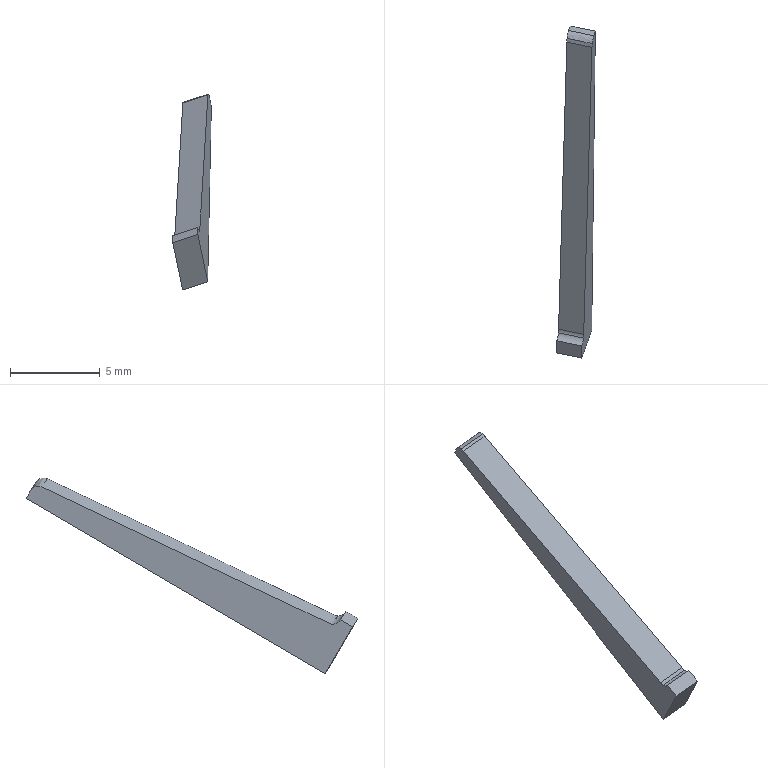Part | STEP file | PN_0037 | 1 solid | 13 faces | box 2.149 x 18.473 x 10.911 mm | volume 52.704 mm3 | plane 7 | spline 6